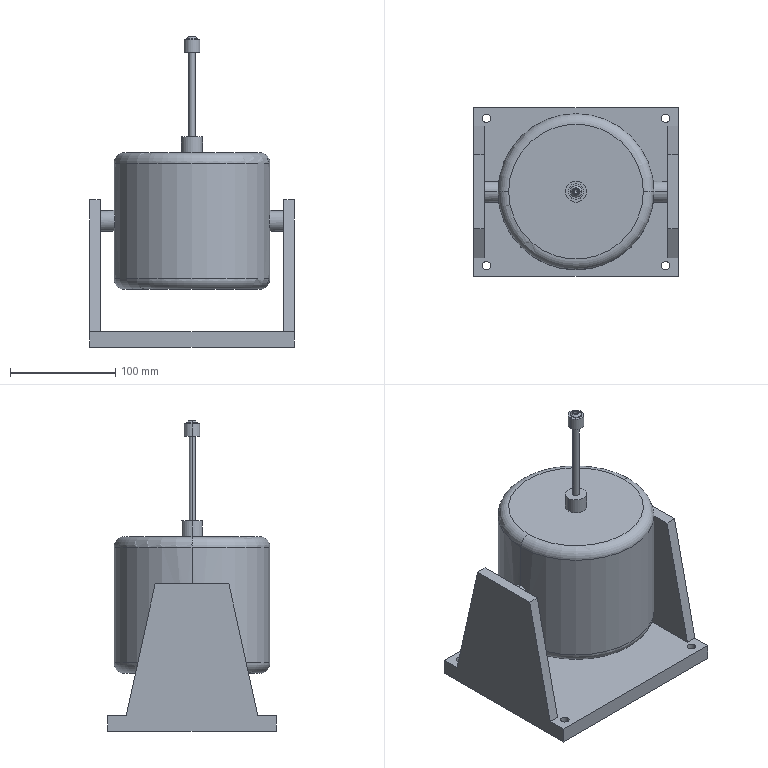Part | SolidWorks | features ICE 7, Chamfer 1, Extrusion 1, Fillet 1, HoleWzd 1, MirrorPattern 1 | 1 solid | 54 faces | box 194.286 x 160 x 295 mm | volume 2941596 mm3 | cylinder 24 | plane 20 | cone 6 | torus 4 | commonest cylinder face diameters 8 x8 20 x6 4.2 x2 6 x2 11 x2 15 x2